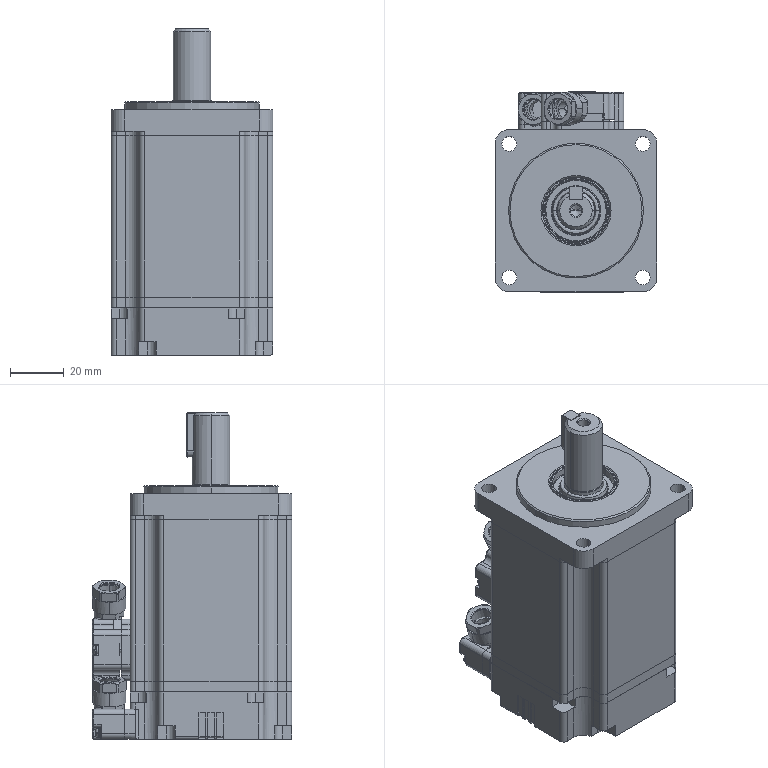Part | SolidWorks | 24 solids | 1737 faces | box 60 x 74.1 x 121 mm | volume 300230 mm3 | plane 985 | cylinder 426 | spline 226 | torus 66 | cone 34 | commonest cylinder face diameters 1 x111 4 x65 10 x38 2 x29 2.2 x24 3.5 x16